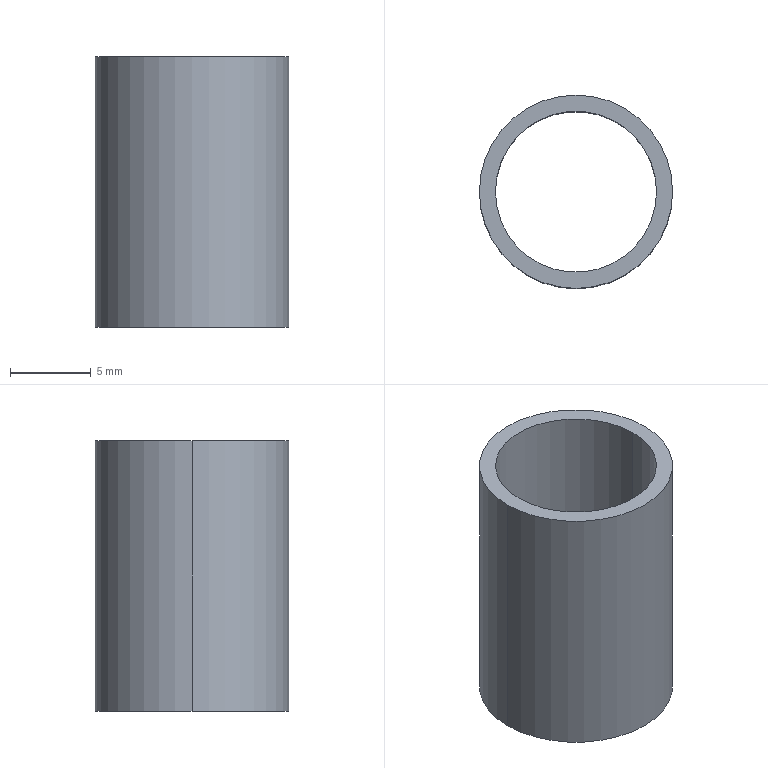Part | SolidWorks | features Extrusion 1 | 1 solid | 6 faces | box 12 x 12 x 16.8 mm | volume 580.566 mm3 | cylinder 4 | plane 2 | commonest cylinder face diameters 10 x2 12 x2
STEP:
#1=CARTESIAN_POINT('',(-5.,0.,8.4));
#2=VERTEX_POINT('',#1);
#3=CARTESIAN_POINT('',(5.,0.,8.4));
#4=VERTEX_POINT('',#3);
#5=CARTESIAN_POINT('',(0.,0.,8.4));
#6=DIRECTION('',(0.,0.,1.));
#7=DIRECTION('',(1.,0.,0.));
#8=AXIS2_PLACEMENT_3D('',#5,#6,#7);
#9=CIRCLE('',#8,5.);
#10=EDGE_CURVE('',#2,#4,#9,.T.);
#11=ORIENTED_EDGE('',*,*,#10,.T.);
#12=CARTESIAN_POINT('',(5.,0.,-8.4));
#13=VERTEX_POINT('',#12);
#14=CARTESIAN_POINT('',(5.,0.,8.4));
#15=DIRECTION('',(0.,0.,-1.));
#16=VECTOR('',#15,1000.);
#17=LINE('',#14,#16);
#18=EDGE_CURVE('',#4,#13,#17,.T.);
#19=ORIENTED_EDGE('',*,*,#18,.T.);
#20=CARTESIAN_POINT('',(-5.,0.,-8.4));
#21=VERTEX_POINT('',#20);
#22=CARTESIAN_POINT('',(0.,0.,-8.4));
#23=DIRECTION('',(0.,0.,1.));
#24=DIRECTION('',(1.,0.,0.));
#25=AXIS2_PLACEMENT_3D('',#22,#23,#24);
#26=CIRCLE('',#25,5.);
#27=EDGE_CURVE('',#21,#13,#26,.T.);
#28=ORIENTED_EDGE('',*,*,#27,.F.);
#29=CARTESIAN_POINT('',(-5.,0.,8.4));
#30=DIRECTION('',(0.,0.,-1.));
#31=VECTOR('',#30,1000.);
#32=LINE('',#29,#31);
#33=EDGE_CURVE('',#2,#21,#32,.T.);
#34=ORIENTED_EDGE('',*,*,#33,.F.);
#35=EDGE_LOOP('',(#11,#19,#28,#34));
#36=FACE_OUTER_BOUND('',#35,.T.);
#37=CARTESIAN_POINT('',(0.,0.,8.4));
#38=DIRECTION('',(0.,0.,-1.));
#39=DIRECTION('',(-1.,0.,0.));
#40=AXIS2_PLACEMENT_3D('',#37,#38,#39);
#41=CYLINDRICAL_SURFACE('',#40,5.);
#42=ADVANCED_FACE('',(#36),#41,.F.);
#43=CARTESIAN_POINT('',(6.,0.,8.4));
#44=VERTEX_POINT('',#43);
#45=CARTESIAN_POINT('',(-6.,0.,8.4));
#46=VERTEX_POINT('',#45);
#47=CARTESIAN_POINT('',(0.,0.,8.4));
#48=DIRECTION('',(0.,0.,1.));
#49=DIRECTION('',(1.,0.,0.));
#50=AXIS2_PLACEMENT_3D('',#47,#48,#49);
#51=CIRCLE('',#50,6.);
#52=EDGE_CURVE('',#44,#46,#51,.T.);
#53=ORIENTED_EDGE('',*,*,#52,.F.);
#54=CARTESIAN_POINT('',(6.,0.,-8.4));
#55=VERTEX_POINT('',#54);
#56=CARTESIAN_POINT('',(6.,0.,8.4));
#57=DIRECTION('',(0.,0.,-1.));
#58=VECTOR('',#57,1000.);
#59=LINE('',#56,#58);
#60=EDGE_CURVE('',#44,#55,#59,.T.);
#61=ORIENTED_EDGE('',*,*,#60,.T.);
#62=CARTESIAN_POINT('',(-6.,0.,-8.4));
#63=VERTEX_POINT('',#62);
#64=CARTESIAN_POINT('',(0.,0.,-8.4));
#65=DIRECTION('',(0.,0.,1.));
#66=DIRECTION('',(1.,0.,0.));
#67=AXIS2_PLACEMENT_3D('',#64,#65,#66);
#68=CIRCLE('',#67,6.);
#69=EDGE_CURVE('',#55,#63,#68,.T.);
#70=ORIENTED_EDGE('',*,*,#69,.T.);
#71=CARTESIAN_POINT('',(-6.,0.,8.4));
#72=DIRECTION('',(0.,0.,-1.));
#73=VECTOR('',#72,1000.);
#74=LINE('',#71,#73);
#75=EDGE_CURVE('',#46,#63,#74,.T.);
#76=ORIENTED_EDGE('',*,*,#75,.F.);
#77=EDGE_LOOP('',(#53,#61,#70,#76));
#78=FACE_OUTER_BOUND('',#77,.T.);
#79=CARTESIAN_POINT('',(0.,0.,8.4));
#80=DIRECTION('',(0.,0.,-1.));
#81=DIRECTION('',(-1.,0.,0.));
#82=AXIS2_PLACEMENT_3D('',#79,#80,#81);
#83=CYLINDRICAL_SURFACE('',#82,6.);
#84=ADVANCED_FACE('',(#78),#83,.T.);
#85=CARTESIAN_POINT('',(0.,0.,8.4));
#86=DIRECTION('',(0.,0.,1.));
#87=DIRECTION('',(1.,0.,0.));
#88=AXIS2_PLACEMENT_3D('',#85,#86,#87);
#89=CIRCLE('',#88,6.);
#90=EDGE_CURVE('',#46,#44,#89,.T.);
#91=ORIENTED_EDGE('',*,*,#90,.T.);
#92=ORIENTED_EDGE('',*,*,#52,.T.);
#93=EDGE_LOOP('',(#91,#92));
#94=FACE_OUTER_BOUND('',#93,.T.);
#95=ORIENTED_EDGE('',*,*,#10,.F.);
#96=CARTESIAN_POINT('',(0.,0.,8.4));
#97=DIRECTION('',(0.,0.,1.));
#98=DIRECTION('',(1.,0.,0.));
#99=AXIS2_PLACEMENT_3D('',#96,#97,#98);
#100=CIRCLE('',#99,5.);
#101=EDGE_CURVE('',#4,#2,#100,.T.);
#102=ORIENTED_EDGE('',*,*,#101,.F.);
#103=EDGE_LOOP('',(#95,#102));
#104=FACE_BOUND('',#103,.T.);
#105=CARTESIAN_POINT('',(0.,0.,8.4));
#106=DIRECTION('',(0.,0.,1.));
#107=DIRECTION('',(1.,0.,0.));
#108=AXIS2_PLACEMENT_3D('',#105,#106,#107);
#109=PLANE('',#108);
#110=ADVANCED_FACE('',(#94,#104),#109,.T.);
#111=CARTESIAN_POINT('',(0.,0.,-8.4));
#112=DIRECTION('',(0.,0.,1.));
#113=DIRECTION('',(1.,0.,0.));
#114=AXIS2_PLACEMENT_3D('',#111,#112,#113);
#115=CIRCLE('',#114,6.);
#116=EDGE_CURVE('',#63,#55,#115,.T.);
#117=ORIENTED_EDGE('',*,*,#116,.F.);
#118=ORIENTED_EDGE('',*,*,#69,.F.);
#119=EDGE_LOOP('',(#117,#118));
#120=FACE_OUTER_BOUND('',#119,.T.);
#121=ORIENTED_EDGE('',*,*,#27,.T.);
#122=CARTESIAN_POINT('',(0.,0.,-8.4));
#123=DIRECTION('',(0.,0.,1.));
#124=DIRECTION('',(1.,0.,0.));
#125=AXIS2_PLACEMENT_3D('',#122,#123,#124);
#126=CIRCLE('',#125,5.);
#127=EDGE_CURVE('',#13,#21,#126,.T.);
#128=ORIENTED_EDGE('',*,*,#127,.T.);
#129=EDGE_LOOP('',(#121,#128));
#130=FACE_BOUND('',#129,.T.);
#131=CARTESIAN_POINT('',(0.,0.,-8.4));
#132=DIRECTION('',(0.,0.,1.));
#133=DIRECTION('',(1.,0.,0.));
#134=AXIS2_PLACEMENT_3D('',#131,#132,#133);
#135=PLANE('',#134);
#136=ADVANCED_FACE('',(#120,#130),#135,.F.);
#137=ORIENTED_EDGE('',*,*,#60,.F.);
#138=ORIENTED_EDGE('',*,*,#90,.F.);
#139=ORIENTED_EDGE('',*,*,#75,.T.);
#140=ORIENTED_EDGE('',*,*,#116,.T.);
#141=EDGE_LOOP('',(#137,#138,#139,#140));
#142=FACE_OUTER_BOUND('',#141,.T.);
#143=CARTESIAN_POINT('',(0.,0.,8.4));
#144=DIRECTION('',(0.,0.,-1.));
#145=DIRECTION('',(-1.,0.,0.));
#146=AXIS2_PLACEMENT_3D('',#143,#144,#145);
#147=CYLINDRICAL_SURFACE('',#146,6.);
#148=ADVANCED_FACE('',(#142),#147,.T.);
#149=ORIENTED_EDGE('',*,*,#18,.F.);
#150=ORIENTED_EDGE('',*,*,#101,.T.);
#151=ORIENTED_EDGE('',*,*,#33,.T.);
#152=ORIENTED_EDGE('',*,*,#127,.F.);
#153=EDGE_LOOP('',(#149,#150,#151,#152));
#154=FACE_OUTER_BOUND('',#153,.T.);
#155=CARTESIAN_POINT('',(0.,0.,8.4));
#156=DIRECTION('',(0.,0.,-1.));
#157=DIRECTION('',(-1.,0.,0.));
#158=AXIS2_PLACEMENT_3D('',#155,#156,#157);
#159=CYLINDRICAL_SURFACE('',#158,5.);
#160=ADVANCED_FACE('',(#154),#159,.F.);
#161=CLOSED_SHELL('',(#42,#84,#110,#136,#148,#160));
#162=MANIFOLD_SOLID_BREP('',#161);
#163=CARTESIAN_POINT('',(0.,0.,0.));
#164=DIRECTION('',(0.,0.,1.));
#165=DIRECTION('',(1.,0.,0.));
#166=AXIS2_PLACEMENT_3D('',#163,#164,#165);
#167=(LENGTH_UNIT()NAMED_UNIT(*)SI_UNIT(.MILLI.,.METRE.));
#168=UNCERTAINTY_MEASURE_WITH_UNIT(LENGTH_MEASURE(0.00001),#167,'','');
#169=(NAMED_UNIT(*)PLANE_ANGLE_UNIT()SI_UNIT($,.RADIAN.));
#170=(NAMED_UNIT(*)SI_UNIT($,.STERADIAN.)SOLID_ANGLE_UNIT());
#171=(GEOMETRIC_REPRESENTATION_CONTEXT(3)GLOBAL_UNCERTAINTY_ASSIGNED_CONTEXT((#168))GLOBAL_UNIT_ASSIGNED_CONTEXT((#167,#169,#170))REPRESENTATION_CONTEXT('',''));
#172=ADVANCED_BREP_SHAPE_REPRESENTATION('',(#162,#166),#171);